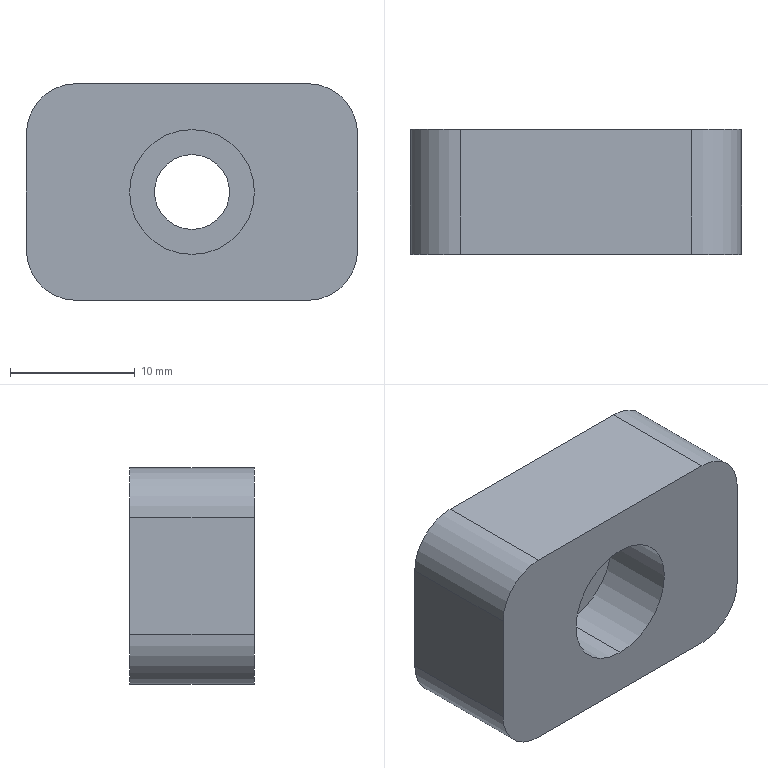Part | STEP file | 1 solid | 15 faces | box 26.5 x 10 x 17.347 mm | volume 3875 mm3 | cylinder 8 | plane 7 | commonest cylinder face diameters 8 x4 6 x2 10 x2
STEP:
#1=CARTESIAN_POINT('',(0.,0.,0.));
#2=DIRECTION('',(0.,0.,1.));
#3=DIRECTION('',(1.,0.,0.));
#4=AXIS2_PLACEMENT_3D('',#1,#2,#3);
#5=CARTESIAN_POINT('',(-93.72,-44.,122.243));
#6=VERTEX_POINT('',#5);
#7=CARTESIAN_POINT('',(-93.72,-40.,122.243));
#8=VERTEX_POINT('',#7);
#9=CARTESIAN_POINT('',(-93.72,-44.,122.243));
#10=DIRECTION('',(0.,1.,0.));
#11=VECTOR('',#10,1.);
#12=LINE('',#9,#11);
#13=CARTESIAN_POINT('',(-93.72,-44.,119.243));
#14=DIRECTION('',(0.,1.,0.));
#15=DIRECTION('',(0.,0.,1.));
#16=AXIS2_PLACEMENT_3D('',#13,#14,#15);
#17=CYLINDRICAL_SURFACE('',#16,3.);
#18=CARTESIAN_POINT('',(6.283,0.));
#19=DIRECTION('',(0.,1.));
#20=VECTOR('',#19,1.);
#21=LINE('',#18,#20);
#22=(GEOMETRIC_REPRESENTATION_CONTEXT(2)PARAMETRIC_REPRESENTATION_CONTEXT()REPRESENTATION_CONTEXT('',''));
#23=DEFINITIONAL_REPRESENTATION('',(#21),#22);
#24=PCURVE('',#17,#23);
#25=CARTESIAN_POINT('',(-93.72,-44.,119.243));
#26=DIRECTION('',(0.,1.,0.));
#27=DIRECTION('',(0.,0.,1.));
#28=AXIS2_PLACEMENT_3D('',#25,#26,#27);
#29=CYLINDRICAL_SURFACE('',#28,3.);
#30=CARTESIAN_POINT('',(0.,0.));
#31=DIRECTION('',(0.,1.));
#32=VECTOR('',#31,1.);
#33=LINE('',#30,#32);
#34=(GEOMETRIC_REPRESENTATION_CONTEXT(2)PARAMETRIC_REPRESENTATION_CONTEXT()REPRESENTATION_CONTEXT('',''));
#35=DEFINITIONAL_REPRESENTATION('',(#33),#34);
#36=PCURVE('',#29,#35);
#37=SURFACE_CURVE('',#12,(#24,#36),.PCURVE_S1.);
#38=EDGE_CURVE('',#6,#8,#37,.T.);
#39=ORIENTED_EDGE('',*,*,#38,.T.);
#40=CARTESIAN_POINT('',(-93.72,-40.,116.243));
#41=VERTEX_POINT('',#40);
#42=CARTESIAN_POINT('',(-93.72,-40.,119.243));
#43=DIRECTION('',(0.,-1.,0.));
#44=DIRECTION('',(0.,0.,-1.));
#45=AXIS2_PLACEMENT_3D('',#42,#43,#44);
#46=CIRCLE('',#45,3.);
#47=CARTESIAN_POINT('',(9.425,4.));
#48=DIRECTION('',(-1.,0.));
#49=VECTOR('',#48,1.);
#50=LINE('',#47,#49);
#51=(GEOMETRIC_REPRESENTATION_CONTEXT(2)PARAMETRIC_REPRESENTATION_CONTEXT()REPRESENTATION_CONTEXT('',''));
#52=DEFINITIONAL_REPRESENTATION('',(#50),#51);
#53=PCURVE('',#17,#52);
#54=CARTESIAN_POINT('',(-93.72,-40.,119.243));
#55=DIRECTION('',(0.,-1.,0.));
#56=DIRECTION('',(0.,0.,-1.));
#57=AXIS2_PLACEMENT_3D('',#54,#55,#56);
#58=PLANE('',#57);
#59=CARTESIAN_POINT('',(0.,0.));
#60=DIRECTION('',(1.,0.));
#61=AXIS2_PLACEMENT_2D('',#59,#60);
#62=CIRCLE('',#61,3.);
#63=(GEOMETRIC_REPRESENTATION_CONTEXT(2)PARAMETRIC_REPRESENTATION_CONTEXT()REPRESENTATION_CONTEXT('',''));
#64=DEFINITIONAL_REPRESENTATION('',(#62),#63);
#65=PCURVE('',#58,#64);
#66=SURFACE_CURVE('',#46,(#53,#65),.PCURVE_S1.);
#67=EDGE_CURVE('',#8,#41,#66,.T.);
#68=ORIENTED_EDGE('',*,*,#67,.T.);
#69=CARTESIAN_POINT('',(-93.72,-44.,116.243));
#70=VERTEX_POINT('',#69);
#71=CARTESIAN_POINT('',(-93.72,-44.,116.243));
#72=DIRECTION('',(0.,1.,0.));
#73=VECTOR('',#72,1.);
#74=LINE('',#71,#73);
#75=CARTESIAN_POINT('',(3.142,0.));
#76=DIRECTION('',(0.,1.));
#77=VECTOR('',#76,1.);
#78=LINE('',#75,#77);
#79=(GEOMETRIC_REPRESENTATION_CONTEXT(2)PARAMETRIC_REPRESENTATION_CONTEXT()REPRESENTATION_CONTEXT('',''));
#80=DEFINITIONAL_REPRESENTATION('',(#78),#79);
#81=PCURVE('',#17,#80);
#82=CARTESIAN_POINT('',(3.142,0.));
#83=DIRECTION('',(0.,1.));
#84=VECTOR('',#83,1.);
#85=LINE('',#82,#84);
#86=(GEOMETRIC_REPRESENTATION_CONTEXT(2)PARAMETRIC_REPRESENTATION_CONTEXT()REPRESENTATION_CONTEXT('',''));
#87=DEFINITIONAL_REPRESENTATION('',(#85),#86);
#88=PCURVE('',#29,#87);
#89=SURFACE_CURVE('',#74,(#81,#88),.PCURVE_S1.);
#90=EDGE_CURVE('',#70,#41,#89,.T.);
#91=ORIENTED_EDGE('',*,*,#90,.F.);
#92=CARTESIAN_POINT('',(-93.72,-44.,119.243));
#93=DIRECTION('',(0.,1.,0.));
#94=DIRECTION('',(0.,0.,1.));
#95=AXIS2_PLACEMENT_3D('',#92,#93,#94);
#96=CIRCLE('',#95,3.);
#97=CARTESIAN_POINT('',(0.,0.));
#98=DIRECTION('',(1.,0.));
#99=VECTOR('',#98,1.);
#100=LINE('',#97,#99);
#101=(GEOMETRIC_REPRESENTATION_CONTEXT(2)PARAMETRIC_REPRESENTATION_CONTEXT()REPRESENTATION_CONTEXT('',''));
#102=DEFINITIONAL_REPRESENTATION('',(#100),#101);
#103=PCURVE('',#17,#102);
#104=CARTESIAN_POINT('',(-93.72,-44.,119.243));
#105=DIRECTION('',(0.,1.,0.));
#106=DIRECTION('',(0.,0.,1.));
#107=AXIS2_PLACEMENT_3D('',#104,#105,#106);
#108=PLANE('',#107);
#109=CARTESIAN_POINT('',(0.,0.));
#110=DIRECTION('',(1.,0.));
#111=AXIS2_PLACEMENT_2D('',#109,#110);
#112=CIRCLE('',#111,3.);
#113=(GEOMETRIC_REPRESENTATION_CONTEXT(2)PARAMETRIC_REPRESENTATION_CONTEXT()REPRESENTATION_CONTEXT('',''));
#114=DEFINITIONAL_REPRESENTATION('',(#112),#113);
#115=PCURVE('',#108,#114);
#116=SURFACE_CURVE('',#96,(#103,#115),.PCURVE_S1.);
#117=EDGE_CURVE('',#70,#6,#116,.T.);
#118=ORIENTED_EDGE('',*,*,#117,.T.);
#119=EDGE_LOOP('',(#39,#68,#91,#118));
#120=FACE_BOUND('',#119,.F.);
#121=ADVANCED_FACE('',(#120),#17,.F.);
#122=CARTESIAN_POINT('',(-93.72,-50.,124.243));
#123=VERTEX_POINT('',#122);
#124=CARTESIAN_POINT('',(-93.72,-44.,124.243));
#125=VERTEX_POINT('',#124);
#126=CARTESIAN_POINT('',(-93.72,-50.,124.243));
#127=DIRECTION('',(0.,1.,0.));
#128=VECTOR('',#127,1.);
#129=LINE('',#126,#128);
#130=CARTESIAN_POINT('',(-93.72,-50.,119.243));
#131=DIRECTION('',(0.,1.,0.));
#132=DIRECTION('',(0.,0.,1.));
#133=AXIS2_PLACEMENT_3D('',#130,#131,#132);
#134=CYLINDRICAL_SURFACE('',#133,5.);
#135=CARTESIAN_POINT('',(6.283,0.));
#136=DIRECTION('',(0.,1.));
#137=VECTOR('',#136,1.);
#138=LINE('',#135,#137);
#139=(GEOMETRIC_REPRESENTATION_CONTEXT(2)PARAMETRIC_REPRESENTATION_CONTEXT()REPRESENTATION_CONTEXT('',''));
#140=DEFINITIONAL_REPRESENTATION('',(#138),#139);
#141=PCURVE('',#134,#140);
#142=CARTESIAN_POINT('',(-93.72,-50.,119.243));
#143=DIRECTION('',(0.,1.,0.));
#144=DIRECTION('',(0.,0.,1.));
#145=AXIS2_PLACEMENT_3D('',#142,#143,#144);
#146=CYLINDRICAL_SURFACE('',#145,5.);
#147=CARTESIAN_POINT('',(0.,0.));
#148=DIRECTION('',(0.,1.));
#149=VECTOR('',#148,1.);
#150=LINE('',#147,#149);
#151=(GEOMETRIC_REPRESENTATION_CONTEXT(2)PARAMETRIC_REPRESENTATION_CONTEXT()REPRESENTATION_CONTEXT('',''));
#152=DEFINITIONAL_REPRESENTATION('',(#150),#151);
#153=PCURVE('',#146,#152);
#154=SURFACE_CURVE('',#129,(#141,#153),.PCURVE_S1.);
#155=EDGE_CURVE('',#123,#125,#154,.T.);
#156=ORIENTED_EDGE('',*,*,#155,.T.);
#157=CARTESIAN_POINT('',(-93.72,-44.,114.243));
#158=VERTEX_POINT('',#157);
#159=CARTESIAN_POINT('',(-93.72,-44.,119.243));
#160=DIRECTION('',(0.,-1.,0.));
#161=DIRECTION('',(0.,0.,-1.));
#162=AXIS2_PLACEMENT_3D('',#159,#160,#161);
#163=CIRCLE('',#162,5.);
#164=CARTESIAN_POINT('',(9.425,6.));
#165=DIRECTION('',(-1.,0.));
#166=VECTOR('',#165,1.);
#167=LINE('',#164,#166);
#168=(GEOMETRIC_REPRESENTATION_CONTEXT(2)PARAMETRIC_REPRESENTATION_CONTEXT()REPRESENTATION_CONTEXT('',''));
#169=DEFINITIONAL_REPRESENTATION('',(#167),#168);
#170=PCURVE('',#134,#169);
#171=CARTESIAN_POINT('',(-5.,0.));
#172=CARTESIAN_POINT('',(-5.,8.66));
#173=CARTESIAN_POINT('',(2.5,4.33));
#174=CARTESIAN_POINT('',(10.,0.));
#175=CARTESIAN_POINT('',(2.5,-4.33));
#176=CARTESIAN_POINT('',(-5.,-8.66));
#177=CARTESIAN_POINT('',(-5.,0.));
#178=(BOUNDED_CURVE()B_SPLINE_CURVE(2,(#171,#172,#173,#174,#175,#176,#177),.UNSPECIFIED.,.T.,.F.)B_SPLINE_CURVE_WITH_KNOTS((1,2,2,2,2,1),(-2.094,0.,2.094,4.189,6.283,8.378),.UNSPECIFIED.)CURVE()GEOMETRIC_REPRESENTATION_ITEM()RATIONAL_B_SPLINE_CURVE((1.,0.5,1.,0.5,1.,0.5,1.))REPRESENTATION_ITEM(''));
#179=(GEOMETRIC_REPRESENTATION_CONTEXT(2)PARAMETRIC_REPRESENTATION_CONTEXT()REPRESENTATION_CONTEXT('',''));
#180=DEFINITIONAL_REPRESENTATION('',(#178),#179);
#181=PCURVE('',#108,#180);
#182=SURFACE_CURVE('',#163,(#170,#181),.PCURVE_S1.);
#183=EDGE_CURVE('',#125,#158,#182,.T.);
#184=ORIENTED_EDGE('',*,*,#183,.T.);
#185=CARTESIAN_POINT('',(-93.72,-50.,114.243));
#186=VERTEX_POINT('',#185);
#187=CARTESIAN_POINT('',(-93.72,-50.,114.243));
#188=DIRECTION('',(0.,1.,0.));
#189=VECTOR('',#188,1.);
#190=LINE('',#187,#189);
#191=CARTESIAN_POINT('',(3.142,0.));
#192=DIRECTION('',(0.,1.));
#193=VECTOR('',#192,1.);
#194=LINE('',#191,#193);
#195=(GEOMETRIC_REPRESENTATION_CONTEXT(2)PARAMETRIC_REPRESENTATION_CONTEXT()REPRESENTATION_CONTEXT('',''));
#196=DEFINITIONAL_REPRESENTATION('',(#194),#195);
#197=PCURVE('',#134,#196);
#198=CARTESIAN_POINT('',(3.142,0.));
#199=DIRECTION('',(0.,1.));
#200=VECTOR('',#199,1.);
#201=LINE('',#198,#200);
#202=(GEOMETRIC_REPRESENTATION_CONTEXT(2)PARAMETRIC_REPRESENTATION_CONTEXT()REPRESENTATION_CONTEXT('',''));
#203=DEFINITIONAL_REPRESENTATION('',(#201),#202);
#204=PCURVE('',#146,#203);
#205=SURFACE_CURVE('',#190,(#197,#204),.PCURVE_S1.);
#206=EDGE_CURVE('',#186,#158,#205,.T.);
#207=ORIENTED_EDGE('',*,*,#206,.F.);
#208=CARTESIAN_POINT('',(-93.72,-50.,119.243));
#209=DIRECTION('',(0.,1.,0.));
#210=DIRECTION('',(0.,0.,1.));
#211=AXIS2_PLACEMENT_3D('',#208,#209,#210);
#212=CIRCLE('',#211,5.);
#213=CARTESIAN_POINT('',(0.,0.));
#214=DIRECTION('',(1.,0.));
#215=VECTOR('',#214,1.);
#216=LINE('',#213,#215);
#217=(GEOMETRIC_REPRESENTATION_CONTEXT(2)PARAMETRIC_REPRESENTATION_CONTEXT()REPRESENTATION_CONTEXT('',''));
#218=DEFINITIONAL_REPRESENTATION('',(#216),#217);
#219=PCURVE('',#134,#218);
#220=CARTESIAN_POINT('',(-93.72,-50.,111.07));
#221=DIRECTION('',(0.,-1.,0.));
#222=DIRECTION('',(0.,0.,-1.));
#223=AXIS2_PLACEMENT_3D('',#220,#221,#222);
#224=PLANE('',#223);
#225=CARTESIAN_POINT('',(-13.173,0.));
#226=CARTESIAN_POINT('',(-13.173,8.66));
#227=CARTESIAN_POINT('',(-5.673,4.33));
#228=CARTESIAN_POINT('',(1.827,0.));
#229=CARTESIAN_POINT('',(-5.673,-4.33));
#230=CARTESIAN_POINT('',(-13.173,-8.66));
#231=CARTESIAN_POINT('',(-13.173,0.));
#232=(BOUNDED_CURVE()B_SPLINE_CURVE(2,(#225,#226,#227,#228,#229,#230,#231),.UNSPECIFIED.,.T.,.F.)B_SPLINE_CURVE_WITH_KNOTS((1,2,2,2,2,1),(-2.094,0.,2.094,4.189,6.283,8.378),.UNSPECIFIED.)CURVE()GEOMETRIC_REPRESENTATION_ITEM()RATIONAL_B_SPLINE_CURVE((1.,0.5,1.,0.5,1.,0.5,1.))REPRESENTATION_ITEM(''));
#233=(GEOMETRIC_REPRESENTATION_CONTEXT(2)PARAMETRIC_REPRESENTATION_CONTEXT()REPRESENTATION_CONTEXT('',''));
#234=DEFINITIONAL_REPRESENTATION('',(#232),#233);
#235=PCURVE('',#224,#234);
#236=SURFACE_CURVE('',#212,(#219,#235),.PCURVE_S1.);
#237=EDGE_CURVE('',#186,#123,#236,.T.);
#238=ORIENTED_EDGE('',*,*,#237,.T.);
#239=EDGE_LOOP('',(#156,#184,#207,#238));
#240=FACE_BOUND('',#239,.F.);
#241=ADVANCED_FACE('',(#240),#134,.F.);
#242=CARTESIAN_POINT('',(-80.47,-40.,114.57));
#243=VERTEX_POINT('',#242);
#244=CARTESIAN_POINT('',(-80.47,-40.,123.916));
#245=VERTEX_POINT('',#244);
#246=CARTESIAN_POINT('',(-80.47,-40.,119.243));
#247=DIRECTION('',(0.,0.,1.));
#248=VECTOR('',#247,1.);
#249=LINE('',#246,#248);
#250=CARTESIAN_POINT('',(-80.47,-50.,119.243));
#251=DIRECTION('',(1.,0.,0.));
#252=DIRECTION('',(0.,0.,-1.));
#253=AXIS2_PLACEMENT_3D('',#250,#251,#252);
#254=PLANE('',#253);
#255=CARTESIAN_POINT('',(0.,10.));
#256=DIRECTION('',(-1.,0.));
#257=VECTOR('',#256,1.);
#258=LINE('',#255,#257);
#259=(GEOMETRIC_REPRESENTATION_CONTEXT(2)PARAMETRIC_REPRESENTATION_CONTEXT()REPRESENTATION_CONTEXT('',''));
#260=DEFINITIONAL_REPRESENTATION('',(#258),#259);
#261=PCURVE('',#254,#260);
#262=CARTESIAN_POINT('',(0.,13.25));
#263=DIRECTION('',(-1.,0.));
#264=VECTOR('',#263,1.);
#265=LINE('',#262,#264);
#266=(GEOMETRIC_REPRESENTATION_CONTEXT(2)PARAMETRIC_REPRESENTATION_CONTEXT()REPRESENTATION_CONTEXT('',''));
#267=DEFINITIONAL_REPRESENTATION('',(#265),#266);
#268=PCURVE('',#58,#267);
#269=SURFACE_CURVE('',#249,(#261,#268),.PCURVE_S1.);
#270=EDGE_CURVE('',#243,#245,#269,.T.);
#271=ORIENTED_EDGE('',*,*,#270,.T.);
#272=CARTESIAN_POINT('',(-80.47,-50.,123.916));
#273=VERTEX_POINT('',#272);
#274=CARTESIAN_POINT('',(-80.47,-50.,123.916));
#275=DIRECTION('',(0.,-1.,0.));
#276=VECTOR('',#275,1.);
#277=LINE('',#274,#276);
#278=CARTESIAN_POINT('',(-4.673,0.));
#279=DIRECTION('',(0.,-1.));
#280=VECTOR('',#279,1.);
#281=LINE('',#278,#280);
#282=(GEOMETRIC_REPRESENTATION_CONTEXT(2)PARAMETRIC_REPRESENTATION_CONTEXT()REPRESENTATION_CONTEXT('',''));
#283=DEFINITIONAL_REPRESENTATION('',(#281),#282);
#284=PCURVE('',#254,#283);
#285=CARTESIAN_POINT('',(-84.47,-42.,123.916));
#286=DIRECTION('',(0.,1.,0.));
#287=DIRECTION('',(0.,0.,1.));
#288=AXIS2_PLACEMENT_3D('',#285,#286,#287);
#289=CYLINDRICAL_SURFACE('',#288,4.);
#290=CARTESIAN_POINT('',(1.571,-8.));
#291=DIRECTION('',(0.,-1.));
#292=VECTOR('',#291,1.);
#293=LINE('',#290,#292);
#294=(GEOMETRIC_REPRESENTATION_CONTEXT(2)PARAMETRIC_REPRESENTATION_CONTEXT()REPRESENTATION_CONTEXT('',''));
#295=DEFINITIONAL_REPRESENTATION('',(#293),#294);
#296=PCURVE('',#289,#295);
#297=SURFACE_CURVE('',#277,(#284,#296),.PCURVE_S1.);
#298=EDGE_CURVE('',#245,#273,#297,.T.);
#299=ORIENTED_EDGE('',*,*,#298,.T.);
#300=CARTESIAN_POINT('',(-80.47,-50.,114.57));
#301=VERTEX_POINT('',#300);
#302=CARTESIAN_POINT('',(-80.47,-50.,111.07));
#303=DIRECTION('',(0.,0.,1.));
#304=VECTOR('',#303,1.);
#305=LINE('',#302,#304);
#306=CARTESIAN_POINT('',(8.173,0.));
#307=DIRECTION('',(-1.,0.));
#308=VECTOR('',#307,1.);
#309=LINE('',#306,#308);
#310=(GEOMETRIC_REPRESENTATION_CONTEXT(2)PARAMETRIC_REPRESENTATION_CONTEXT()REPRESENTATION_CONTEXT('',''));
#311=DEFINITIONAL_REPRESENTATION('',(#309),#310);
#312=PCURVE('',#254,#311);
#313=CARTESIAN_POINT('',(0.,13.25));
#314=DIRECTION('',(-1.,0.));
#315=VECTOR('',#314,1.);
#316=LINE('',#313,#315);
#317=(GEOMETRIC_REPRESENTATION_CONTEXT(2)PARAMETRIC_REPRESENTATION_CONTEXT()REPRESENTATION_CONTEXT('',''));
#318=DEFINITIONAL_REPRESENTATION('',(#316),#317);
#319=PCURVE('',#224,#318);
#320=SURFACE_CURVE('',#305,(#312,#319),.PCURVE_S1.);
#321=EDGE_CURVE('',#301,#273,#320,.T.);
#322=ORIENTED_EDGE('',*,*,#321,.F.);
#323=CARTESIAN_POINT('',(-80.47,-50.,114.57));
#324=DIRECTION('',(0.,1.,0.));
#325=VECTOR('',#324,1.);
#326=LINE('',#323,#325);
#327=CARTESIAN_POINT('',(4.673,0.));
#328=DIRECTION('',(0.,1.));
#329=VECTOR('',#328,1.);
#330=LINE('',#327,#329);
#331=(GEOMETRIC_REPRESENTATION_CONTEXT(2)PARAMETRIC_REPRESENTATION_CONTEXT()REPRESENTATION_CONTEXT('',''));
#332=DEFINITIONAL_REPRESENTATION('',(#330),#331);
#333=PCURVE('',#254,#332);
#334=CARTESIAN_POINT('',(-84.47,-42.,114.57));
#335=DIRECTION('',(0.,-1.,0.));
#336=DIRECTION('',(0.,0.,-1.));
#337=AXIS2_PLACEMENT_3D('',#334,#335,#336);
#338=CYLINDRICAL_SURFACE('',#337,4.);
#339=CARTESIAN_POINT('',(1.571,8.));
#340=DIRECTION('',(0.,-1.));
#341=VECTOR('',#340,1.);
#342=LINE('',#339,#341);
#343=(GEOMETRIC_REPRESENTATION_CONTEXT(2)PARAMETRIC_REPRESENTATION_CONTEXT()REPRESENTATION_CONTEXT('',''));
#344=DEFINITIONAL_REPRESENTATION('',(#342),#343);
#345=PCURVE('',#338,#344);
#346=SURFACE_CURVE('',#326,(#333,#345),.PCURVE_S1.);
#347=EDGE_CURVE('',#301,#243,#346,.T.);
#348=ORIENTED_EDGE('',*,*,#347,.T.);
#349=EDGE_LOOP('',(#271,#299,#322,#348));
#350=FACE_BOUND('',#349,.T.);
#351=ADVANCED_FACE('',(#350),#254,.T.);
#352=ORIENTED_EDGE('',*,*,#67,.T.);
#353=CARTESIAN_POINT('',(-93.72,-40.,119.243));
#354=DIRECTION('',(0.,-1.,0.));
#355=DIRECTION('',(0.,0.,-1.));
#356=AXIS2_PLACEMENT_3D('',#353,#354,#355);
#357=CIRCLE('',#356,3.);
#358=CARTESIAN_POINT('',(0.,0.));
#359=DIRECTION('',(1.,0.));
#360=AXIS2_PLACEMENT_2D('',#358,#359);
#361=CIRCLE('',#360,3.);
#362=(GEOMETRIC_REPRESENTATION_CONTEXT(2)PARAMETRIC_REPRESENTATION_CONTEXT()REPRESENTATION_CONTEXT('',''));
#363=DEFINITIONAL_REPRESENTATION('',(#361),#362);
#364=PCURVE('',#58,#363);
#365=CARTESIAN_POINT('',(3.142,4.));
#366=DIRECTION('',(-1.,0.));
#367=VECTOR('',#366,1.);
#368=LINE('',#365,#367);
#369=(GEOMETRIC_REPRESENTATION_CONTEXT(2)PARAMETRIC_REPRESENTATION_CONTEXT()REPRESENTATION_CONTEXT('',''));
#370=DEFINITIONAL_REPRESENTATION('',(#368),#369);
#371=PCURVE('',#29,#370);
#372=SURFACE_CURVE('',#357,(#364,#371),.PCURVE_S1.);
#373=EDGE_CURVE('',#41,#8,#372,.T.);
#374=ORIENTED_EDGE('',*,*,#373,.T.);
#375=EDGE_LOOP('',(#352,#374));
#376=FACE_BOUND('',#375,.T.);
#377=CARTESIAN_POINT('',(-102.97,-40.,127.916));
#378=VERTEX_POINT('',#377);
#379=CARTESIAN_POINT('',(-84.47,-40.,127.916));
#380=VERTEX_POINT('',#379);
#381=CARTESIAN_POINT('',(-93.72,-40.,127.916));
#382=DIRECTION('',(1.,0.,0.));
#383=VECTOR('',#382,1.);
#384=LINE('',#381,#383);
#385=CARTESIAN_POINT('',(-8.673,0.));
#386=DIRECTION('',(0.,1.));
#387=VECTOR('',#386,1.);
#388=LINE('',#385,#387);
#389=(GEOMETRIC_REPRESENTATION_CONTEXT(2)PARAMETRIC_REPRESENTATION_CONTEXT()REPRESENTATION_CONTEXT('',''));
#390=DEFINITIONAL_REPRESENTATION('',(#388),#389);
#391=PCURVE('',#58,#390);
#392=CARTESIAN_POINT('',(-93.72,-42.,127.916));
#393=DIRECTION('',(0.,0.,1.));
#394=DIRECTION('',(1.,0.,0.));
#395=AXIS2_PLACEMENT_3D('',#392,#393,#394);
#396=PLANE('',#395);
#397=CARTESIAN_POINT('',(0.,2.));
#398=DIRECTION('',(1.,0.));
#399=VECTOR('',#398,1.);
#400=LINE('',#397,#399);
#401=(GEOMETRIC_REPRESENTATION_CONTEXT(2)PARAMETRIC_REPRESENTATION_CONTEXT()REPRESENTATION_CONTEXT('',''));
#402=DEFINITIONAL_REPRESENTATION('',(#400),#401);
#403=PCURVE('',#396,#402);
#404=SURFACE_CURVE('',#384,(#391,#403),.PCURVE_S1.);
#405=EDGE_CURVE('',#378,#380,#404,.T.);
#406=ORIENTED_EDGE('',*,*,#405,.T.);
#407=CARTESIAN_POINT('',(-84.47,-40.,123.916));
#408=DIRECTION('',(0.,1.,0.));
#409=DIRECTION('',(0.,0.,-1.));
#410=AXIS2_PLACEMENT_3D('',#407,#408,#409);
#411=CIRCLE('',#410,4.);
#412=CARTESIAN_POINT('',(-0.6733,9.25));
#413=CARTESIAN_POINT('',(-0.6733,2.322));
#414=CARTESIAN_POINT('',(-6.673,5.786));
#415=CARTESIAN_POINT('',(-12.673,9.25));
#416=CARTESIAN_POINT('',(-6.673,12.714));
#417=CARTESIAN_POINT('',(-0.6733,16.178));
#418=CARTESIAN_POINT('',(-0.6733,9.25));
#419=(BOUNDED_CURVE()B_SPLINE_CURVE(2,(#412,#413,#414,#415,#416,#417,#418),.UNSPECIFIED.,.T.,.F.)B_SPLINE_CURVE_WITH_KNOTS((1,2,2,2,2,1),(-2.094,0.,2.094,4.189,6.283,8.378),.UNSPECIFIED.)CURVE()GEOMETRIC_REPRESENTATION_ITEM()RATIONAL_B_SPLINE_CURVE((1.,0.5,1.,0.5,1.,0.5,1.))REPRESENTATION_ITEM(''));
#420=(GEOMETRIC_REPRESENTATION_CONTEXT(2)PARAMETRIC_REPRESENTATION_CONTEXT()REPRESENTATION_CONTEXT('',''));
#421=DEFINITIONAL_REPRESENTATION('',(#419),#420);
#422=PCURVE('',#58,#421);
#423=CARTESIAN_POINT('',(-3.142,2.));
#424=DIRECTION('',(1.,0.));
#425=VECTOR('',#424,1.);
#426=LINE('',#423,#425);
#427=(GEOMETRIC_REPRESENTATION_CONTEXT(2)PARAMETRIC_REPRESENTATION_CONTEXT()REPRESENTATION_CONTEXT('',''));
#428=DEFINITIONAL_REPRESENTATION('',(#426),#427);
#429=PCURVE('',#289,#428);
#430=SURFACE_CURVE('',#411,(#422,#429),.PCURVE_S1.);
#431=EDGE_CURVE('',#380,#245,#430,.T.);
#432=ORIENTED_EDGE('',*,*,#431,.T.);
#433=ORIENTED_EDGE('',*,*,#270,.F.);
#434=CARTESIAN_POINT('',(-84.47,-40.,110.57));
#435=VERTEX_POINT('',#434);
#436=CARTESIAN_POINT('',(-84.47,-40.,114.57));
#437=DIRECTION('',(0.,1.,0.));
#438=DIRECTION('',(0.,0.,-1.));
#439=AXIS2_PLACEMENT_3D('',#436,#437,#438);
#440=CIRCLE('',#439,4.);
#441=CARTESIAN_POINT('',(8.673,9.25));
#442=CARTESIAN_POINT('',(8.673,2.322));
#443=CARTESIAN_POINT('',(2.673,5.786));
#444=CARTESIAN_POINT('',(-3.327,9.25));
#445=CARTESIAN_POINT('',(2.673,12.714));
#446=CARTESIAN_POINT('',(8.673,16.178));
#447=CARTESIAN_POINT('',(8.673,9.25));
#448=(BOUNDED_CURVE()B_SPLINE_CURVE(2,(#441,#442,#443,#444,#445,#446,#447),.UNSPECIFIED.,.T.,.F.)B_SPLINE_CURVE_WITH_KNOTS((1,2,2,2,2,1),(-2.094,0.,2.094,4.189,6.283,8.378),.UNSPECIFIED.)CURVE()GEOMETRIC_REPRESENTATION_ITEM()RATIONAL_B_SPLINE_CURVE((1.,0.5,1.,0.5,1.,0.5,1.))REPRESENTATION_ITEM(''));
#449=(GEOMETRIC_REPRESENTATION_CONTEXT(2)PARAMETRIC_REPRESENTATION_CONTEXT()REPRESENTATION_CONTEXT('',''));
#450=DEFINITIONAL_REPRESENTATION('',(#448),#449);
#451=PCURVE('',#58,#450);
#452=CARTESIAN_POINT('',(6.283,-2.));
#453=DIRECTION('',(-1.,0.));
#454=VECTOR('',#453,1.);
#455=LINE('',#452,#454);
#456=(GEOMETRIC_REPRESENTATION_CONTEXT(2)PARAMETRIC_REPRESENTATION_CONTEXT()REPRESENTATION_CONTEXT('',''));
#457=DEFINITIONAL_REPRESENTATION('',(#455),#456);
#458=PCURVE('',#338,#457);
#459=SURFACE_CURVE('',#440,(#451,#458),.PCURVE_S1.);
#460=EDGE_CURVE('',#243,#435,#459,.T.);
#461=ORIENTED_EDGE('',*,*,#460,.T.);
#462=CARTESIAN_POINT('',(-102.97,-40.,110.57));
#463=VERTEX_POINT('',#462);
#464=CARTESIAN_POINT('',(-93.72,-40.,110.57));
#465=DIRECTION('',(-1.,0.,0.));
#466=VECTOR('',#465,1.);
#467=LINE('',#464,#466);
#468=CARTESIAN_POINT('',(8.673,0.));
#469=DIRECTION('',(0.,-1.));
#470=VECTOR('',#469,1.);
#471=LINE('',#468,#470);
#472=(GEOMETRIC_REPRESENTATION_CONTEXT(2)PARAMETRIC_REPRESENTATION_CONTEXT()REPRESENTATION_CONTEXT('',''));
#473=DEFINITIONAL_REPRESENTATION('',(#471),#472);
#474=PCURVE('',#58,#473);
#475=CARTESIAN_POINT('',(-93.72,-42.,110.57));
#476=DIRECTION('',(0.,0.,-1.));
#477=DIRECTION('',(-1.,0.,0.));
#478=AXIS2_PLACEMENT_3D('',#475,#476,#477);
#479=PLANE('',#478);
#480=CARTESIAN_POINT('',(0.,2.));
#481=DIRECTION('',(1.,0.));
#482=VECTOR('',#481,1.);
#483=LINE('',#480,#482);
#484=(GEOMETRIC_REPRESENTATION_CONTEXT(2)PARAMETRIC_REPRESENTATION_CONTEXT()REPRESENTATION_CONTEXT('',''));
#485=DEFINITIONAL_REPRESENTATION('',(#483),#484);
#486=PCURVE('',#479,#485);
#487=SURFACE_CURVE('',#467,(#474,#486),.PCURVE_S1.);
#488=EDGE_CURVE('',#435,#463,#487,.T.);
#489=ORIENTED_EDGE('',*,*,#488,.T.);
#490=CARTESIAN_POINT('',(-106.97,-40.,114.57));
#491=VERTEX_POINT('',#490);
#492=CARTESIAN_POINT('',(-102.97,-40.,114.57));
#493=DIRECTION('',(0.,1.,0.));
#494=DIRECTION('',(0.,0.,-1.));
#495=AXIS2_PLACEMENT_3D('',#492,#493,#494);
#496=CIRCLE('',#495,4.);
#497=CARTESIAN_POINT('',(8.673,-9.25));
#498=CARTESIAN_POINT('',(8.673,-16.178));
#499=CARTESIAN_POINT('',(2.673,-12.714));
#500=CARTESIAN_POINT('',(-3.327,-9.25));
#501=CARTESIAN_POINT('',(2.673,-5.786));
#502=CARTESIAN_POINT('',(8.673,-2.322));
#503=CARTESIAN_POINT('',(8.673,-9.25));
#504=(BOUNDED_CURVE()B_SPLINE_CURVE(2,(#497,#498,#499,#500,#501,#502,#503),.UNSPECIFIED.,.T.,.F.)B_SPLINE_CURVE_WITH_KNOTS((1,2,2,2,2,1),(-2.094,0.,2.094,4.189,6.283,8.378),.UNSPECIFIED.)CURVE()GEOMETRIC_REPRESENTATION_ITEM()RATIONAL_B_SPLINE_CURVE((1.,0.5,1.,0.5,1.,0.5,1.))REPRESENTATION_ITEM(''));
#505=(GEOMETRIC_REPRESENTATION_CONTEXT(2)PARAMETRIC_REPRESENTATION_CONTEXT()REPRESENTATION_CONTEXT('',''));
#506=DEFINITIONAL_REPRESENTATION('',(#504),#505);
#507=PCURVE('',#58,#506);
#508=CARTESIAN_POINT('',(-102.97,-50.,114.57));
#509=DIRECTION('',(0.,1.,0.));
#510=DIRECTION('',(0.,0.,1.));
#511=AXIS2_PLACEMENT_3D('',#508,#509,#510);
#512=CYLINDRICAL_SURFACE('',#511,4.);
#513=CARTESIAN_POINT('',(3.142,10.));
#514=DIRECTION('',(1.,0.));
#515=VECTOR('',#514,1.);
#516=LINE('',#513,#515);
#517=(GEOMETRIC_REPRESENTATION_CONTEXT(2)PARAMETRIC_REPRESENTATION_CONTEXT()REPRESENTATION_CONTEXT('',''));
#518=DEFINITIONAL_REPRESENTATION('',(#516),#517);
#519=PCURVE('',#512,#518);
#520=SURFACE_CURVE('',#496,(#507,#519),.PCURVE_S1.);
#521=EDGE_CURVE('',#463,#491,#520,.T.);
#522=ORIENTED_EDGE('',*,*,#521,.T.);
#523=CARTESIAN_POINT('',(-106.97,-40.,123.916));
#524=VERTEX_POINT('',#523);
#525=CARTESIAN_POINT('',(-106.97,-40.,119.243));
#526=DIRECTION('',(0.,0.,1.));
#527=VECTOR('',#526,1.);
#528=LINE('',#525,#527);
#529=CARTESIAN_POINT('',(0.,-13.25));
#530=DIRECTION('',(-1.,0.));
#531=VECTOR('',#530,1.);
#532=LINE('',#529,#531);
#533=(GEOMETRIC_REPRESENTATION_CONTEXT(2)PARAMETRIC_REPRESENTATION_CONTEXT()REPRESENTATION_CONTEXT('',''));
#534=DEFINITIONAL_REPRESENTATION('',(#532),#533);
#535=PCURVE('',#58,#534);
#536=CARTESIAN_POINT('',(-106.97,-50.,119.243));
#537=DIRECTION('',(1.,0.,0.));
#538=DIRECTION('',(0.,0.,-1.));
#539=AXIS2_PLACEMENT_3D('',#536,#537,#538);
#540=PLANE('',#539);
#541=CARTESIAN_POINT('',(0.,10.));
#542=DIRECTION('',(-1.,0.));
#543=VECTOR('',#542,1.);
#544=LINE('',#541,#543);
#545=(GEOMETRIC_REPRESENTATION_CONTEXT(2)PARAMETRIC_REPRESENTATION_CONTEXT()REPRESENTATION_CONTEXT('',''));
#546=DEFINITIONAL_REPRESENTATION('',(#544),#545);
#547=PCURVE('',#540,#546);
#548=SURFACE_CURVE('',#528,(#535,#547),.PCURVE_S1.);
#549=EDGE_CURVE('',#491,#524,#548,.T.);
#550=ORIENTED_EDGE('',*,*,#549,.T.);
#551=CARTESIAN_POINT('',(-102.97,-40.,123.916));
#552=DIRECTION('',(0.,1.,0.));
#553=DIRECTION('',(0.,0.,-1.));
#554=AXIS2_PLACEMENT_3D('',#551,#552,#553);
#555=CIRCLE('',#554,4.);
#556=CARTESIAN_POINT('',(-0.6733,-9.25));
#557=CARTESIAN_POINT('',(-0.6733,-16.178));
#558=CARTESIAN_POINT('',(-6.673,-12.714));
#559=CARTESIAN_POINT('',(-12.673,-9.25));
#560=CARTESIAN_POINT('',(-6.673,-5.786));
#561=CARTESIAN_POINT('',(-0.6733,-2.322));
#562=CARTESIAN_POINT('',(-0.6733,-9.25));
#563=(BOUNDED_CURVE()B_SPLINE_CURVE(2,(#556,#557,#558,#559,#560,#561,#562),.UNSPECIFIED.,.T.,.F.)B_SPLINE_CURVE_WITH_KNOTS((1,2,2,2,2,1),(-2.094,0.,2.094,4.189,6.283,8.378),.UNSPECIFIED.)CURVE()GEOMETRIC_REPRESENTATION_ITEM()RATIONAL_B_SPLINE_CURVE((1.,0.5,1.,0.5,1.,0.5,1.))REPRESENTATION_ITEM(''));
#564=(GEOMETRIC_REPRESENTATION_CONTEXT(2)PARAMETRIC_REPRESENTATION_CONTEXT()REPRESENTATION_CONTEXT('',''));
#565=DEFINITIONAL_REPRESENTATION('',(#563),#564);
#566=PCURVE('',#58,#565);
#567=CARTESIAN_POINT('',(-102.97,-50.,123.916));
#568=DIRECTION('',(0.,-1.,0.));
#569=DIRECTION('',(0.,0.,-1.));
#570=AXIS2_PLACEMENT_3D('',#567,#568,#569);
#571=CYLINDRICAL_SURFACE('',#570,4.);
#572=CARTESIAN_POINT('',(6.283,-10.));
#573=DIRECTION('',(-1.,0.));
#574=VECTOR('',#573,1.);
#575=LINE('',#572,#574);
#576=(GEOMETRIC_REPRESENTATION_CONTEXT(2)PARAMETRIC_REPRESENTATION_CONTEXT()REPRESENTATION_CONTEXT('',''));
#577=DEFINITIONAL_REPRESENTATION('',(#575),#576);
#578=PCURVE('',#571,#577);
#579=SURFACE_CURVE('',#555,(#566,#578),.PCURVE_S1.);
#580=EDGE_CURVE('',#524,#378,#579,.T.);
#581=ORIENTED_EDGE('',*,*,#580,.T.);
#582=EDGE_LOOP('',(#406,#432,#433,#461,#489,#522,#550,#581));
#583=FACE_BOUND('',#582,.T.);
#584=ADVANCED_FACE('',(#376,#583),#58,.F.);
#585=ORIENTED_EDGE('',*,*,#488,.F.);
#586=CARTESIAN_POINT('',(-84.47,-50.,110.57));
#587=VERTEX_POINT('',#586);
#588=CARTESIAN_POINT('',(-84.47,-42.,110.57));
#589=DIRECTION('',(0.,-1.,0.));
#590=VECTOR('',#589,1.);
#591=LINE('',#588,#590);
#592=CARTESIAN_POINT('',(-9.25,0.));
#593=DIRECTION('',(0.,-1.));
#594=VECTOR('',#593,1.);
#595=LINE('',#592,#594);
#596=(GEOMETRIC_REPRESENTATION_CONTEXT(2)PARAMETRIC_REPRESENTATION_CONTEXT()REPRESENTATION_CONTEXT('',''));
#597=DEFINITIONAL_REPRESENTATION('',(#595),#596);
#598=PCURVE('',#479,#597);
#599=CARTESIAN_POINT('',(0.,0.));
#600=DIRECTION('',(0.,1.));
#601=VECTOR('',#600,1.);
#602=LINE('',#599,#601);
#603=(GEOMETRIC_REPRESENTATION_CONTEXT(2)PARAMETRIC_REPRESENTATION_CONTEXT()REPRESENTATION_CONTEXT('',''));
#604=DEFINITIONAL_REPRESENTATION('',(#602),#603);
#605=PCURVE('',#338,#604);
#606=SURFACE_CURVE('',#591,(#598,#605),.PCURVE_S1.);
#607=EDGE_CURVE('',#435,#587,#606,.T.);
#608=ORIENTED_EDGE('',*,*,#607,.T.);
#609=CARTESIAN_POINT('',(-102.97,-50.,110.57));
#610=VERTEX_POINT('',#609);
#611=CARTESIAN_POINT('',(-93.72,-50.,110.57));
#612=DIRECTION('',(1.,0.,0.));
#613=VECTOR('',#612,1.);
#614=LINE('',#611,#613);
#615=CARTESIAN_POINT('',(0.,-8.));
#616=DIRECTION('',(-1.,0.));
#617=VECTOR('',#616,1.);
#618=LINE('',#615,#617);
#619=(GEOMETRIC_REPRESENTATION_CONTEXT(2)PARAMETRIC_REPRESENTATION_CONTEXT()REPRESENTATION_CONTEXT('',''));
#620=DEFINITIONAL_REPRESENTATION('',(#618),#619);
#621=PCURVE('',#479,#620);
#622=CARTESIAN_POINT('',(0.5,0.));
#623=DIRECTION('',(0.,1.));
#624=VECTOR('',#623,1.);
#625=LINE('',#622,#624);
#626=(GEOMETRIC_REPRESENTATION_CONTEXT(2)PARAMETRIC_REPRESENTATION_CONTEXT()REPRESENTATION_CONTEXT('',''));
#627=DEFINITIONAL_REPRESENTATION('',(#625),#626);
#628=PCURVE('',#224,#627);
#629=SURFACE_CURVE('',#614,(#621,#628),.PCURVE_S1.);
#630=EDGE_CURVE('',#610,#587,#629,.T.);
#631=ORIENTED_EDGE('',*,*,#630,.F.);
#632=CARTESIAN_POINT('',(-102.97,-40.,110.57));
#633=DIRECTION('',(0.,1.,0.));
#634=VECTOR('',#633,1.);
#635=LINE('',#632,#634);
#636=CARTESIAN_POINT('',(9.25,2.));
#637=DIRECTION('',(0.,1.));
#638=VECTOR('',#637,1.);
#639=LINE('',#636,#638);
#640=(GEOMETRIC_REPRESENTATION_CONTEXT(2)PARAMETRIC_REPRESENTATION_CONTEXT()REPRESENTATION_CONTEXT('',''));
#641=DEFINITIONAL_REPRESENTATION('',(#639),#640);
#642=PCURVE('',#479,#641);
#643=CARTESIAN_POINT('',(3.142,10.));
#644=DIRECTION('',(0.,1.));
#645=VECTOR('',#644,1.);
#646=LINE('',#643,#645);
#647=(GEOMETRIC_REPRESENTATION_CONTEXT(2)PARAMETRIC_REPRESENTATION_CONTEXT()REPRESENTATION_CONTEXT('',''));
#648=DEFINITIONAL_REPRESENTATION('',(#646),#647);
#649=PCURVE('',#512,#648);
#650=SURFACE_CURVE('',#635,(#642,#649),.PCURVE_S1.);
#651=EDGE_CURVE('',#610,#463,#650,.T.);
#652=ORIENTED_EDGE('',*,*,#651,.T.);
#653=EDGE_LOOP('',(#585,#608,#631,#652));
#654=FACE_BOUND('',#653,.T.);
#655=ADVANCED_FACE('',(#654),#479,.T.);
#656=CARTESIAN_POINT('',(-93.72,-50.,119.243));
#657=DIRECTION('',(0.,1.,0.));
#658=DIRECTION('',(0.,0.,1.));
#659=AXIS2_PLACEMENT_3D('',#656,#657,#658);
#660=CIRCLE('',#659,5.);
#661=CARTESIAN_POINT('',(-13.173,0.));
#662=CARTESIAN_POINT('',(-13.173,8.66));
#663=CARTESIAN_POINT('',(-5.673,4.33));
#664=CARTESIAN_POINT('',(1.827,0.));
#665=CARTESIAN_POINT('',(-5.673,-4.33));
#666=CARTESIAN_POINT('',(-13.173,-8.66));
#667=CARTESIAN_POINT('',(-13.173,0.));
#668=(BOUNDED_CURVE()B_SPLINE_CURVE(2,(#661,#662,#663,#664,#665,#666,#667),.UNSPECIFIED.,.T.,.F.)B_SPLINE_CURVE_WITH_KNOTS((1,2,2,2,2,1),(-2.094,0.,2.094,4.189,6.283,8.378),.UNSPECIFIED.)CURVE()GEOMETRIC_REPRESENTATION_ITEM()RATIONAL_B_SPLINE_CURVE((1.,0.5,1.,0.5,1.,0.5,1.))REPRESENTATION_ITEM(''));
#669=(GEOMETRIC_REPRESENTATION_CONTEXT(2)PARAMETRIC_REPRESENTATION_CONTEXT()REPRESENTATION_CONTEXT('',''));
#670=DEFINITIONAL_REPRESENTATION('',(#668),#669);
#671=PCURVE('',#224,#670);
#672=CARTESIAN_POINT('',(0.,0.));
#673=DIRECTION('',(1.,0.));
#674=VECTOR('',#673,1.);
#675=LINE('',#672,#674);
#676=(GEOMETRIC_REPRESENTATION_CONTEXT(2)PARAMETRIC_REPRESENTATION_CONTEXT()REPRESENTATION_CONTEXT('',''));
#677=DEFINITIONAL_REPRESENTATION('',(#675),#676);
#678=PCURVE('',#146,#677);
#679=SURFACE_CURVE('',#660,(#671,#678),.PCURVE_S1.);
#680=EDGE_CURVE('',#123,#186,#679,.T.);
#681=ORIENTED_EDGE('',*,*,#680,.T.);
#682=ORIENTED_EDGE('',*,*,#237,.T.);
#683=EDGE_LOOP('',(#681,#682));
#684=FACE_BOUND('',#683,.T.);
#685=ORIENTED_EDGE('',*,*,#321,.T.);
#686=CARTESIAN_POINT('',(-84.47,-50.,127.916));
#687=VERTEX_POINT('',#686);
#688=CARTESIAN_POINT('',(-84.47,-50.,123.916));
#689=DIRECTION('',(0.,-1.,0.));
#690=DIRECTION('',(0.,0.,-1.));
#691=AXIS2_PLACEMENT_3D('',#688,#689,#690);
#692=CIRCLE('',#691,4.);
#693=CARTESIAN_POINT('',(-12.847,9.25));
#694=DIRECTION('',(1.,0.));
#695=AXIS2_PLACEMENT_2D('',#693,#694);
#696=CIRCLE('',#695,4.);
#697=(GEOMETRIC_REPRESENTATION_CONTEXT(2)PARAMETRIC_REPRESENTATION_CONTEXT()REPRESENTATION_CONTEXT('',''));
#698=DEFINITIONAL_REPRESENTATION('',(#696),#697);
#699=PCURVE('',#224,#698);
#700=CARTESIAN_POINT('',(3.142,-8.));
#701=DIRECTION('',(-1.,0.));
#702=VECTOR('',#701,1.);
#703=LINE('',#700,#702);
#704=(GEOMETRIC_REPRESENTATION_CONTEXT(2)PARAMETRIC_REPRESENTATION_CONTEXT()REPRESENTATION_CONTEXT('',''));
#705=DEFINITIONAL_REPRESENTATION('',(#703),#704);
#706=PCURVE('',#289,#705);
#707=SURFACE_CURVE('',#692,(#699,#706),.PCURVE_S1.);
#708=EDGE_CURVE('',#273,#687,#707,.T.);
#709=ORIENTED_EDGE('',*,*,#708,.T.);
#710=CARTESIAN_POINT('',(-102.97,-50.,127.916));
#711=VERTEX_POINT('',#710);
#712=CARTESIAN_POINT('',(-93.72,-50.,127.916));
#713=DIRECTION('',(-1.,0.,0.));
#714=VECTOR('',#713,1.);
#715=LINE('',#712,#714);
#716=CARTESIAN_POINT('',(-16.846,0.));
#717=DIRECTION('',(0.,-1.));
#718=VECTOR('',#717,1.);
#719=LINE('',#716,#718);
#720=(GEOMETRIC_REPRESENTATION_CONTEXT(2)PARAMETRIC_REPRESENTATION_CONTEXT()REPRESENTATION_CONTEXT('',''));
#721=DEFINITIONAL_REPRESENTATION('',(#719),#720);
#722=PCURVE('',#224,#721);
#723=CARTESIAN_POINT('',(0.,-8.));
#724=DIRECTION('',(-1.,0.));
#725=VECTOR('',#724,1.);
#726=LINE('',#723,#725);
#727=(GEOMETRIC_REPRESENTATION_CONTEXT(2)PARAMETRIC_REPRESENTATION_CONTEXT()REPRESENTATION_CONTEXT('',''));
#728=DEFINITIONAL_REPRESENTATION('',(#726),#727);
#729=PCURVE('',#396,#728);
#730=SURFACE_CURVE('',#715,(#722,#729),.PCURVE_S1.);
#731=EDGE_CURVE('',#687,#711,#730,.T.);
#732=ORIENTED_EDGE('',*,*,#731,.T.);
#733=CARTESIAN_POINT('',(-106.97,-50.,123.916));
#734=VERTEX_POINT('',#733);
#735=CARTESIAN_POINT('',(-102.97,-50.,123.916));
#736=DIRECTION('',(0.,-1.,0.));
#737=DIRECTION('',(0.,0.,-1.));
#738=AXIS2_PLACEMENT_3D('',#735,#736,#737);
#739=CIRCLE('',#738,4.);
#740=CARTESIAN_POINT('',(-12.847,-9.25));
#741=DIRECTION('',(1.,0.));
#742=AXIS2_PLACEMENT_2D('',#740,#741);
#743=CIRCLE('',#742,4.);
#744=(GEOMETRIC_REPRESENTATION_CONTEXT(2)PARAMETRIC_REPRESENTATION_CONTEXT()REPRESENTATION_CONTEXT('',''));
#745=DEFINITIONAL_REPRESENTATION('',(#743),#744);
#746=PCURVE('',#224,#745);
#747=CARTESIAN_POINT('',(0.,0.));
#748=DIRECTION('',(1.,0.));
#749=VECTOR('',#748,1.);
#750=LINE('',#747,#749);
#751=(GEOMETRIC_REPRESENTATION_CONTEXT(2)PARAMETRIC_REPRESENTATION_CONTEXT()REPRESENTATION_CONTEXT('',''));
#752=DEFINITIONAL_REPRESENTATION('',(#750),#751);
#753=PCURVE('',#571,#752);
#754=SURFACE_CURVE('',#739,(#746,#753),.PCURVE_S1.);
#755=EDGE_CURVE('',#711,#734,#754,.T.);
#756=ORIENTED_EDGE('',*,*,#755,.T.);
#757=CARTESIAN_POINT('',(-106.97,-50.,114.57));
#758=VERTEX_POINT('',#757);
#759=CARTESIAN_POINT('',(-106.97,-50.,111.07));
#760=DIRECTION('',(0.,0.,1.));
#761=VECTOR('',#760,1.);
#762=LINE('',#759,#761);
#763=CARTESIAN_POINT('',(0.,-13.25));
#764=DIRECTION('',(-1.,0.));
#765=VECTOR('',#764,1.);
#766=LINE('',#763,#765);
#767=(GEOMETRIC_REPRESENTATION_CONTEXT(2)PARAMETRIC_REPRESENTATION_CONTEXT()REPRESENTATION_CONTEXT('',''));
#768=DEFINITIONAL_REPRESENTATION('',(#766),#767);
#769=PCURVE('',#224,#768);
#770=CARTESIAN_POINT('',(8.173,0.));
#771=DIRECTION('',(-1.,0.));
#772=VECTOR('',#771,1.);
#773=LINE('',#770,#772);
#774=(GEOMETRIC_REPRESENTATION_CONTEXT(2)PARAMETRIC_REPRESENTATION_CONTEXT()REPRESENTATION_CONTEXT('',''));
#775=DEFINITIONAL_REPRESENTATION('',(#773),#774);
#776=PCURVE('',#540,#775);
#777=SURFACE_CURVE('',#762,(#769,#776),.PCURVE_S1.);
#778=EDGE_CURVE('',#758,#734,#777,.T.);
#779=ORIENTED_EDGE('',*,*,#778,.F.);
#780=CARTESIAN_POINT('',(-102.97,-50.,114.57));
#781=DIRECTION('',(0.,-1.,0.));
#782=DIRECTION('',(0.,0.,-1.));
#783=AXIS2_PLACEMENT_3D('',#780,#781,#782);
#784=CIRCLE('',#783,4.);
#785=CARTESIAN_POINT('',(-3.5,-9.25));
#786=DIRECTION('',(1.,0.));
#787=AXIS2_PLACEMENT_2D('',#785,#786);
#788=CIRCLE('',#787,4.);
#789=(GEOMETRIC_REPRESENTATION_CONTEXT(2)PARAMETRIC_REPRESENTATION_CONTEXT()REPRESENTATION_CONTEXT('',''));
#790=DEFINITIONAL_REPRESENTATION('',(#788),#789);
#791=PCURVE('',#224,#790);
#792=CARTESIAN_POINT('',(9.425,0.));
#793=DIRECTION('',(-1.,0.));
#794=VECTOR('',#793,1.);
#795=LINE('',#792,#794);
#796=(GEOMETRIC_REPRESENTATION_CONTEXT(2)PARAMETRIC_REPRESENTATION_CONTEXT()REPRESENTATION_CONTEXT('',''));
#797=DEFINITIONAL_REPRESENTATION('',(#795),#796);
#798=PCURVE('',#512,#797);
#799=SURFACE_CURVE('',#784,(#791,#798),.PCURVE_S1.);
#800=EDGE_CURVE('',#758,#610,#799,.T.);
#801=ORIENTED_EDGE('',*,*,#800,.T.);
#802=ORIENTED_EDGE('',*,*,#630,.T.);
#803=CARTESIAN_POINT('',(-84.47,-50.,114.57));
#804=DIRECTION('',(0.,-1.,0.));
#805=DIRECTION('',(0.,0.,-1.));
#806=AXIS2_PLACEMENT_3D('',#803,#804,#805);
#807=CIRCLE('',#806,4.);
#808=CARTESIAN_POINT('',(-3.5,9.25));
#809=DIRECTION('',(1.,0.));
#810=AXIS2_PLACEMENT_2D('',#808,#809);
#811=CIRCLE('',#810,4.);
#812=(GEOMETRIC_REPRESENTATION_CONTEXT(2)PARAMETRIC_REPRESENTATION_CONTEXT()REPRESENTATION_CONTEXT('',''));
#813=DEFINITIONAL_REPRESENTATION('',(#811),#812);
#814=PCURVE('',#224,#813);
#815=CARTESIAN_POINT('',(0.,8.));
#816=DIRECTION('',(1.,0.));
#817=VECTOR('',#816,1.);
#818=LINE('',#815,#817);
#819=(GEOMETRIC_REPRESENTATION_CONTEXT(2)PARAMETRIC_REPRESENTATION_CONTEXT()REPRESENTATION_CONTEXT('',''));
#820=DEFINITIONAL_REPRESENTATION('',(#818),#819);
#821=PCURVE('',#338,#820);
#822=SURFACE_CURVE('',#807,(#814,#821),.PCURVE_S1.);
#823=EDGE_CURVE('',#587,#301,#822,.T.);
#824=ORIENTED_EDGE('',*,*,#823,.T.);
#825=EDGE_LOOP('',(#685,#709,#732,#756,#779,#801,#802,#824));
#826=FACE_BOUND('',#825,.T.);
#827=ADVANCED_FACE('',(#684,#826),#224,.T.);
#828=ORIENTED_EDGE('',*,*,#731,.F.);
#829=CARTESIAN_POINT('',(-84.47,-42.,127.916));
#830=DIRECTION('',(0.,1.,0.));
#831=VECTOR('',#830,1.);
#832=LINE('',#829,#831);
#833=CARTESIAN_POINT('',(9.25,0.));
#834=DIRECTION('',(0.,1.));
#835=VECTOR('',#834,1.);
#836=LINE('',#833,#835);
#837=(GEOMETRIC_REPRESENTATION_CONTEXT(2)PARAMETRIC_REPRESENTATION_CONTEXT()REPRESENTATION_CONTEXT('',''));
#838=DEFINITIONAL_REPRESENTATION('',(#836),#837);
#839=PCURVE('',#396,#838);
#840=CARTESIAN_POINT('',(0.,0.));
#841=DIRECTION('',(0.,1.));
#842=VECTOR('',#841,1.);
#843=LINE('',#840,#842);
#844=(GEOMETRIC_REPRESENTATION_CONTEXT(2)PARAMETRIC_REPRESENTATION_CONTEXT()REPRESENTATION_CONTEXT('',''));
#845=DEFINITIONAL_REPRESENTATION('',(#843),#844);
#846=PCURVE('',#289,#845);
#847=SURFACE_CURVE('',#832,(#839,#846),.PCURVE_S1.);
#848=EDGE_CURVE('',#687,#380,#847,.T.);
#849=ORIENTED_EDGE('',*,*,#848,.T.);
#850=ORIENTED_EDGE('',*,*,#405,.F.);
#851=CARTESIAN_POINT('',(-102.97,-50.,127.916));
#852=DIRECTION('',(0.,-1.,0.));
#853=VECTOR('',#852,1.);
#854=LINE('',#851,#853);
#855=CARTESIAN_POINT('',(-9.25,-8.));
#856=DIRECTION('',(0.,-1.));
#857=VECTOR('',#856,1.);
#858=LINE('',#855,#857);
#859=(GEOMETRIC_REPRESENTATION_CONTEXT(2)PARAMETRIC_REPRESENTATION_CONTEXT()REPRESENTATION_CONTEXT('',''));
#860=DEFINITIONAL_REPRESENTATION('',(#858),#859);
#861=PCURVE('',#396,#860);
#862=CARTESIAN_POINT('',(3.142,0.));
#863=DIRECTION('',(0.,1.));
#864=VECTOR('',#863,1.);
#865=LINE('',#862,#864);
#866=(GEOMETRIC_REPRESENTATION_CONTEXT(2)PARAMETRIC_REPRESENTATION_CONTEXT()REPRESENTATION_CONTEXT('',''));
#867=DEFINITIONAL_REPRESENTATION('',(#865),#866);
#868=PCURVE('',#571,#867);
#869=SURFACE_CURVE('',#854,(#861,#868),.PCURVE_S1.);
#870=EDGE_CURVE('',#378,#711,#869,.T.);
#871=ORIENTED_EDGE('',*,*,#870,.T.);
#872=EDGE_LOOP('',(#828,#849,#850,#871));
#873=FACE_BOUND('',#872,.T.);
#874=ADVANCED_FACE('',(#873),#396,.T.);
#875=ORIENTED_EDGE('',*,*,#549,.F.);
#876=CARTESIAN_POINT('',(-106.97,-50.,114.57));
#877=DIRECTION('',(0.,-1.,0.));
#878=VECTOR('',#877,1.);
#879=LINE('',#876,#878);
#880=CARTESIAN_POINT('',(4.673,0.));
#881=DIRECTION('',(0.,-1.));
#882=VECTOR('',#881,1.);
#883=LINE('',#880,#882);
#884=(GEOMETRIC_REPRESENTATION_CONTEXT(2)PARAMETRIC_REPRESENTATION_CONTEXT()REPRESENTATION_CONTEXT('',''));
#885=DEFINITIONAL_REPRESENTATION('',(#883),#884);
#886=PCURVE('',#540,#885);
#887=CARTESIAN_POINT('',(4.712,0.));
#888=DIRECTION('',(0.,-1.));
#889=VECTOR('',#888,1.);
#890=LINE('',#887,#889);
#891=(GEOMETRIC_REPRESENTATION_CONTEXT(2)PARAMETRIC_REPRESENTATION_CONTEXT()REPRESENTATION_CONTEXT('',''));
#892=DEFINITIONAL_REPRESENTATION('',(#890),#891);
#893=PCURVE('',#512,#892);
#894=SURFACE_CURVE('',#879,(#886,#893),.PCURVE_S1.);
#895=EDGE_CURVE('',#491,#758,#894,.T.);
#896=ORIENTED_EDGE('',*,*,#895,.T.);
#897=ORIENTED_EDGE('',*,*,#778,.T.);
#898=CARTESIAN_POINT('',(-106.97,-40.,123.916));
#899=DIRECTION('',(0.,1.,0.));
#900=VECTOR('',#899,1.);
#901=LINE('',#898,#900);
#902=CARTESIAN_POINT('',(-4.673,10.));
#903=DIRECTION('',(0.,1.));
#904=VECTOR('',#903,1.);
#905=LINE('',#902,#904);
#906=(GEOMETRIC_REPRESENTATION_CONTEXT(2)PARAMETRIC_REPRESENTATION_CONTEXT()REPRESENTATION_CONTEXT('',''));
#907=DEFINITIONAL_REPRESENTATION('',(#905),#906);
#908=PCURVE('',#540,#907);
#909=CARTESIAN_POINT('',(4.712,-10.));
#910=DIRECTION('',(0.,-1.));
#911=VECTOR('',#910,1.);
#912=LINE('',#909,#911);
#913=(GEOMETRIC_REPRESENTATION_CONTEXT(2)PARAMETRIC_REPRESENTATION_CONTEXT()REPRESENTATION_CONTEXT('',''));
#914=DEFINITIONAL_REPRESENTATION('',(#912),#913);
#915=PCURVE('',#571,#914);
#916=SURFACE_CURVE('',#901,(#908,#915),.PCURVE_S1.);
#917=EDGE_CURVE('',#734,#524,#916,.T.);
#918=ORIENTED_EDGE('',*,*,#917,.T.);
#919=EDGE_LOOP('',(#875,#896,#897,#918));
#920=FACE_BOUND('',#919,.T.);
#921=ADVANCED_FACE('',(#920),#540,.F.);
#922=ORIENTED_EDGE('',*,*,#708,.F.);
#923=ORIENTED_EDGE('',*,*,#298,.F.);
#924=ORIENTED_EDGE('',*,*,#431,.F.);
#925=ORIENTED_EDGE('',*,*,#848,.F.);
#926=EDGE_LOOP('',(#922,#923,#924,#925));
#927=FACE_BOUND('',#926,.T.);
#928=ADVANCED_FACE('',(#927),#289,.T.);
#929=ORIENTED_EDGE('',*,*,#460,.F.);
#930=ORIENTED_EDGE('',*,*,#347,.F.);
#931=ORIENTED_EDGE('',*,*,#823,.F.);
#932=ORIENTED_EDGE('',*,*,#607,.F.);
#933=EDGE_LOOP('',(#929,#930,#931,#932));
#934=FACE_BOUND('',#933,.T.);
#935=ADVANCED_FACE('',(#934),#338,.T.);
#936=ORIENTED_EDGE('',*,*,#521,.F.);
#937=ORIENTED_EDGE('',*,*,#651,.F.);
#938=ORIENTED_EDGE('',*,*,#800,.F.);
#939=ORIENTED_EDGE('',*,*,#895,.F.);
#940=EDGE_LOOP('',(#936,#937,#938,#939));
#941=FACE_BOUND('',#940,.T.);
#942=ADVANCED_FACE('',(#941),#512,.T.);
#943=ORIENTED_EDGE('',*,*,#755,.F.);
#944=ORIENTED_EDGE('',*,*,#870,.F.);
#945=ORIENTED_EDGE('',*,*,#580,.F.);
#946=ORIENTED_EDGE('',*,*,#917,.F.);
#947=EDGE_LOOP('',(#943,#944,#945,#946));
#948=FACE_BOUND('',#947,.T.);
#949=ADVANCED_FACE('',(#948),#571,.T.);
#950=CARTESIAN_POINT('',(-93.72,-44.,119.243));
#951=DIRECTION('',(0.,1.,0.));
#952=DIRECTION('',(0.,0.,1.));
#953=AXIS2_PLACEMENT_3D('',#950,#951,#952);
#954=CIRCLE('',#953,3.);
#955=CARTESIAN_POINT('',(0.,0.));
#956=DIRECTION('',(1.,0.));
#957=AXIS2_PLACEMENT_2D('',#955,#956);
#958=CIRCLE('',#957,3.);
#959=(GEOMETRIC_REPRESENTATION_CONTEXT(2)PARAMETRIC_REPRESENTATION_CONTEXT()REPRESENTATION_CONTEXT('',''));
#960=DEFINITIONAL_REPRESENTATION('',(#958),#959);
#961=PCURVE('',#108,#960);
#962=CARTESIAN_POINT('',(0.,0.));
#963=DIRECTION('',(1.,0.));
#964=VECTOR('',#963,1.);
#965=LINE('',#962,#964);
#966=(GEOMETRIC_REPRESENTATION_CONTEXT(2)PARAMETRIC_REPRESENTATION_CONTEXT()REPRESENTATION_CONTEXT('',''));
#967=DEFINITIONAL_REPRESENTATION('',(#965),#966);
#968=PCURVE('',#29,#967);
#969=SURFACE_CURVE('',#954,(#961,#968),.PCURVE_S1.);
#970=EDGE_CURVE('',#6,#70,#969,.T.);
#971=ORIENTED_EDGE('',*,*,#970,.T.);
#972=ORIENTED_EDGE('',*,*,#117,.T.);
#973=EDGE_LOOP('',(#971,#972));
#974=FACE_BOUND('',#973,.T.);
#975=ORIENTED_EDGE('',*,*,#183,.T.);
#976=CARTESIAN_POINT('',(-93.72,-44.,119.243));
#977=DIRECTION('',(0.,-1.,0.));
#978=DIRECTION('',(0.,0.,-1.));
#979=AXIS2_PLACEMENT_3D('',#976,#977,#978);
#980=CIRCLE('',#979,5.);
#981=CARTESIAN_POINT('',(-5.,0.));
#982=CARTESIAN_POINT('',(-5.,8.66));
#983=CARTESIAN_POINT('',(2.5,4.33));
#984=CARTESIAN_POINT('',(10.,0.));
#985=CARTESIAN_POINT('',(2.5,-4.33));
#986=CARTESIAN_POINT('',(-5.,-8.66));
#987=CARTESIAN_POINT('',(-5.,0.));
#988=(BOUNDED_CURVE()B_SPLINE_CURVE(2,(#981,#982,#983,#984,#985,#986,#987),.UNSPECIFIED.,.T.,.F.)B_SPLINE_CURVE_WITH_KNOTS((1,2,2,2,2,1),(-2.094,0.,2.094,4.189,6.283,8.378),.UNSPECIFIED.)CURVE()GEOMETRIC_REPRESENTATION_ITEM()RATIONAL_B_SPLINE_CURVE((1.,0.5,1.,0.5,1.,0.5,1.))REPRESENTATION_ITEM(''));
#989=(GEOMETRIC_REPRESENTATION_CONTEXT(2)PARAMETRIC_REPRESENTATION_CONTEXT()REPRESENTATION_CONTEXT('',''));
#990=DEFINITIONAL_REPRESENTATION('',(#988),#989);
#991=PCURVE('',#108,#990);
#992=CARTESIAN_POINT('',(3.142,6.));
#993=DIRECTION('',(-1.,0.));
#994=VECTOR('',#993,1.);
#995=LINE('',#992,#994);
#996=(GEOMETRIC_REPRESENTATION_CONTEXT(2)PARAMETRIC_REPRESENTATION_CONTEXT()REPRESENTATION_CONTEXT('',''));
#997=DEFINITIONAL_REPRESENTATION('',(#995),#996);
#998=PCURVE('',#146,#997);
#999=SURFACE_CURVE('',#980,(#991,#998),.PCURVE_S1.);
#1000=EDGE_CURVE('',#158,#125,#999,.T.);
#1001=ORIENTED_EDGE('',*,*,#1000,.T.);
#1002=EDGE_LOOP('',(#975,#1001));
#1003=FACE_BOUND('',#1002,.T.);
#1004=ADVANCED_FACE('',(#974,#1003),#108,.F.);
#1005=ORIENTED_EDGE('',*,*,#1000,.T.);
#1006=ORIENTED_EDGE('',*,*,#155,.F.);
#1007=ORIENTED_EDGE('',*,*,#680,.T.);
#1008=ORIENTED_EDGE('',*,*,#206,.T.);
#1009=EDGE_LOOP('',(#1005,#1006,#1007,#1008));
#1010=FACE_BOUND('',#1009,.F.);
#1011=ADVANCED_FACE('',(#1010),#146,.F.);
#1012=ORIENTED_EDGE('',*,*,#373,.T.);
#1013=ORIENTED_EDGE('',*,*,#38,.F.);
#1014=ORIENTED_EDGE('',*,*,#970,.T.);
#1015=ORIENTED_EDGE('',*,*,#90,.T.);
#1016=EDGE_LOOP('',(#1012,#1013,#1014,#1015));
#1017=FACE_BOUND('',#1016,.F.);
#1018=ADVANCED_FACE('',(#1017),#29,.F.);
#1019=CLOSED_SHELL('',(#121,#241,#351,#584,#655,#827,#874,#921,#928,#935,#942,#949,#1004,#1011,#1018));
#1020=MANIFOLD_SOLID_BREP('',#1019);
#1021=(LENGTH_UNIT()NAMED_UNIT(*)SI_UNIT(.MILLI.,.METRE.));
#1022=UNCERTAINTY_MEASURE_WITH_UNIT(LENGTH_MEASURE(0.0000001),#1021,'','');
#1023=(NAMED_UNIT(*)PLANE_ANGLE_UNIT()SI_UNIT($,.RADIAN.));
#1024=(NAMED_UNIT(*)SI_UNIT($,.STERADIAN.)SOLID_ANGLE_UNIT());
#1025=(GEOMETRIC_REPRESENTATION_CONTEXT(3)GLOBAL_UNCERTAINTY_ASSIGNED_CONTEXT((#1022))GLOBAL_UNIT_ASSIGNED_CONTEXT((#1021,#1023,#1024))REPRESENTATION_CONTEXT('',''));
#1026=ADVANCED_BREP_SHAPE_REPRESENTATION('',(#4,#1020),#1025);